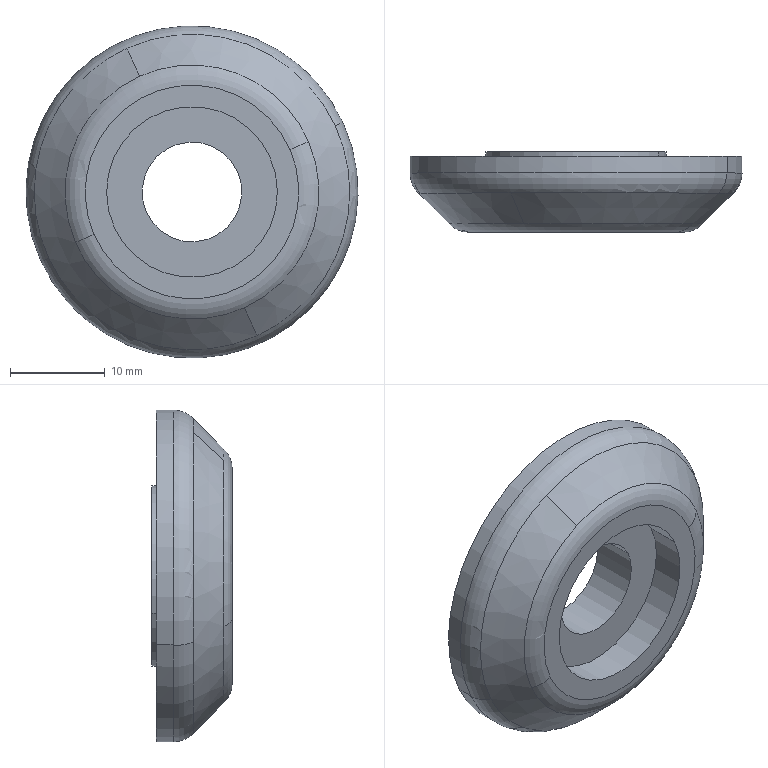Part | SolidWorks | features BaseBody 1 | 1 solid | 18 faces | box 35 x 8.5 x 35 mm | volume 5235 mm3 | cylinder 8 | torus 4 | plane 4 | cone 2 | commonest cylinder face diameters 10.5 x2 18 x2 19 x2 35 x2
STEP:
#1=CARTESIAN_POINT('',(-397.851,-130.5,38.987));
#2=VERTEX_POINT('',#1);
#3=CARTESIAN_POINT('',(-377.198,-130.5,47.953));
#4=VERTEX_POINT('',#3);
#5=CARTESIAN_POINT('',(-387.524,-130.5,43.47));
#6=DIRECTION('',(0.,-1.,0.));
#7=DIRECTION('',(-0.9114,0.,-0.4115));
#8=AXIS2_PLACEMENT_3D('',#5,#6,#7);
#9=CIRCLE('',#8,11.257);
#10=EDGE_CURVE('',#2,#4,#9,.T.);
#11=ORIENTED_EDGE('',*,*,#10,.F.);
#12=CARTESIAN_POINT('',(-399.797,-129.621,38.143));
#13=VERTEX_POINT('',#12);
#14=CARTESIAN_POINT('',(-397.851,-127.5,38.987));
#15=DIRECTION('',(0.3982,0.,-0.9173));
#16=DIRECTION('',(-0.9173,0.,-0.3982));
#17=AXIS2_PLACEMENT_3D('',#14,#15,#16);
#18=CIRCLE('',#17,3.);
#19=EDGE_CURVE('',#2,#13,#18,.T.);
#20=ORIENTED_EDGE('',*,*,#19,.T.);
#21=CARTESIAN_POINT('',(-382.019,-129.621,31.277));
#22=VERTEX_POINT('',#21);
#23=CARTESIAN_POINT('',(-387.524,-129.621,43.47));
#24=DIRECTION('',(0.,-1.,0.));
#25=DIRECTION('',(-0.9114,0.,-0.4115));
#26=AXIS2_PLACEMENT_3D('',#23,#24,#25);
#27=CIRCLE('',#26,13.379);
#28=EDGE_CURVE('',#13,#22,#27,.T.);
#29=ORIENTED_EDGE('',*,*,#28,.T.);
#30=CARTESIAN_POINT('',(-375.252,-129.621,48.797));
#31=VERTEX_POINT('',#30);
#32=CARTESIAN_POINT('',(-387.524,-129.621,43.47));
#33=DIRECTION('',(0.,-1.,0.));
#34=DIRECTION('',(-0.9114,0.,-0.4115));
#35=AXIS2_PLACEMENT_3D('',#32,#33,#34);
#36=CIRCLE('',#35,13.379);
#37=EDGE_CURVE('',#22,#31,#36,.T.);
#38=ORIENTED_EDGE('',*,*,#37,.T.);
#39=CARTESIAN_POINT('',(-377.198,-127.5,47.953));
#40=DIRECTION('',(-0.3982,0.,0.9173));
#41=DIRECTION('',(0.9173,0.,0.3982));
#42=AXIS2_PLACEMENT_3D('',#39,#40,#41);
#43=CIRCLE('',#42,3.);
#44=EDGE_CURVE('',#4,#31,#43,.T.);
#45=ORIENTED_EDGE('',*,*,#44,.F.);
#46=EDGE_LOOP('',(#11,#20,#29,#38,#45));
#47=FACE_OUTER_BOUND('',#46,.T.);
#48=CARTESIAN_POINT('',(-387.524,-127.5,43.47));
#49=DIRECTION('',(0.,1.,0.));
#50=DIRECTION('',(0.9173,0.,0.3982));
#51=AXIS2_PLACEMENT_3D('',#48,#49,#50);
#52=TOROIDAL_SURFACE('',#51,11.257,3.);
#53=ADVANCED_FACE('',(#47),#52,.T.);
#54=ORIENTED_EDGE('',*,*,#37,.F.);
#55=CARTESIAN_POINT('',(-380.685,-126.379,28.321));
#56=VERTEX_POINT('',#55);
#57=CARTESIAN_POINT('',(-381.352,-128.,29.799));
#58=DIRECTION('',(0.291,0.7071,-0.6445));
#59=VECTOR('',#58,1000.);
#60=LINE('',#57,#59);
#61=EDGE_CURVE('',#22,#56,#60,.T.);
#62=ORIENTED_EDGE('',*,*,#61,.T.);
#63=CARTESIAN_POINT('',(-372.434,-126.379,50.438));
#64=VERTEX_POINT('',#63);
#65=CARTESIAN_POINT('',(-387.524,-126.379,43.47));
#66=DIRECTION('',(0.,1.,0.));
#67=DIRECTION('',(-0.9114,0.,-0.4115));
#68=AXIS2_PLACEMENT_3D('',#65,#66,#67);
#69=CIRCLE('',#68,16.621);
#70=EDGE_CURVE('',#64,#56,#69,.T.);
#71=ORIENTED_EDGE('',*,*,#70,.F.);
#72=CARTESIAN_POINT('',(-394.364,-126.379,58.619));
#73=VERTEX_POINT('',#72);
#74=CARTESIAN_POINT('',(-387.524,-126.379,43.47));
#75=DIRECTION('',(0.,1.,0.));
#76=DIRECTION('',(-0.9114,0.,-0.4115));
#77=AXIS2_PLACEMENT_3D('',#74,#75,#76);
#78=CIRCLE('',#77,16.621);
#79=EDGE_CURVE('',#73,#64,#78,.T.);
#80=ORIENTED_EDGE('',*,*,#79,.F.);
#81=CARTESIAN_POINT('',(-393.03,-129.621,55.663));
#82=VERTEX_POINT('',#81);
#83=CARTESIAN_POINT('',(-393.697,-128.,57.141));
#84=DIRECTION('',(-0.291,0.7071,0.6445));
#85=VECTOR('',#84,1000.);
#86=LINE('',#83,#85);
#87=EDGE_CURVE('',#82,#73,#86,.T.);
#88=ORIENTED_EDGE('',*,*,#87,.F.);
#89=CARTESIAN_POINT('',(-387.524,-129.621,43.47));
#90=DIRECTION('',(0.,-1.,0.));
#91=DIRECTION('',(-0.9114,0.,-0.4115));
#92=AXIS2_PLACEMENT_3D('',#89,#90,#91);
#93=CIRCLE('',#92,13.379);
#94=EDGE_CURVE('',#31,#82,#93,.T.);
#95=ORIENTED_EDGE('',*,*,#94,.F.);
#96=EDGE_LOOP('',(#54,#62,#71,#80,#88,#95));
#97=FACE_OUTER_BOUND('',#96,.T.);
#98=CARTESIAN_POINT('',(-387.524,-128.,43.47));
#99=DIRECTION('',(0.,1.,0.));
#100=DIRECTION('',(-0.4115,0.,0.9114));
#101=AXIS2_PLACEMENT_3D('',#98,#99,#100);
#102=CONICAL_SURFACE('',#101,15.,0.7854);
#103=ADVANCED_FACE('',(#97),#102,.T.);
#104=CARTESIAN_POINT('',(-371.636,-124.257,50.806));
#105=VERTEX_POINT('',#104);
#106=CARTESIAN_POINT('',(-371.575,-124.257,50.672));
#107=VERTEX_POINT('',#106);
#108=CARTESIAN_POINT('',(-387.524,-124.257,43.47));
#109=DIRECTION('',(0.,1.,0.));
#110=DIRECTION('',(0.9114,0.,0.4115));
#111=AXIS2_PLACEMENT_3D('',#108,#109,#110);
#112=CIRCLE('',#111,17.5);
#113=EDGE_CURVE('',#105,#107,#112,.T.);
#114=ORIENTED_EDGE('',*,*,#113,.F.);
#115=CARTESIAN_POINT('',(-374.36,-124.257,49.548));
#116=DIRECTION('',(0.4192,0.,-0.9079));
#117=DIRECTION('',(-0.9079,0.,-0.4192));
#118=AXIS2_PLACEMENT_3D('',#115,#116,#117);
#119=CIRCLE('',#118,3.);
#120=EDGE_CURVE('',#105,#64,#119,.T.);
#121=ORIENTED_EDGE('',*,*,#120,.T.);
#122=ORIENTED_EDGE('',*,*,#70,.T.);
#123=CARTESIAN_POINT('',(-402.615,-126.379,36.502));
#124=VERTEX_POINT('',#123);
#125=CARTESIAN_POINT('',(-387.524,-126.379,43.47));
#126=DIRECTION('',(0.,1.,0.));
#127=DIRECTION('',(-0.9114,0.,-0.4115));
#128=AXIS2_PLACEMENT_3D('',#125,#126,#127);
#129=CIRCLE('',#128,16.621);
#130=EDGE_CURVE('',#56,#124,#129,.T.);
#131=ORIENTED_EDGE('',*,*,#130,.T.);
#132=CARTESIAN_POINT('',(-403.413,-124.257,36.134));
#133=VERTEX_POINT('',#132);
#134=CARTESIAN_POINT('',(-400.689,-124.257,37.392));
#135=DIRECTION('',(-0.4192,0.,0.9079));
#136=DIRECTION('',(0.9079,0.,0.4192));
#137=AXIS2_PLACEMENT_3D('',#134,#135,#136);
#138=CIRCLE('',#137,3.);
#139=EDGE_CURVE('',#133,#124,#138,.T.);
#140=ORIENTED_EDGE('',*,*,#139,.F.);
#141=CARTESIAN_POINT('',(-387.524,-124.257,43.47));
#142=DIRECTION('',(0.,1.,0.));
#143=DIRECTION('',(0.9114,0.,0.4115));
#144=AXIS2_PLACEMENT_3D('',#141,#142,#143);
#145=CIRCLE('',#144,17.5);
#146=EDGE_CURVE('',#107,#133,#145,.T.);
#147=ORIENTED_EDGE('',*,*,#146,.F.);
#148=EDGE_LOOP('',(#114,#121,#122,#131,#140,#147));
#149=FACE_OUTER_BOUND('',#148,.T.);
#150=CARTESIAN_POINT('',(-387.524,-124.257,43.47));
#151=DIRECTION('',(0.,-1.,0.));
#152=DIRECTION('',(-0.9079,0.,-0.4192));
#153=AXIS2_PLACEMENT_3D('',#150,#151,#152);
#154=TOROIDAL_SURFACE('',#153,14.5,3.);
#155=ADVANCED_FACE('',(#149),#154,.T.);
#156=CARTESIAN_POINT('',(-392.309,-122.,41.31));
#157=VERTEX_POINT('',#156);
#158=CARTESIAN_POINT('',(-382.74,-122.,45.631));
#159=VERTEX_POINT('',#158);
#160=CARTESIAN_POINT('',(-387.524,-122.,43.47));
#161=DIRECTION('',(0.,1.,0.));
#162=DIRECTION('',(-0.9114,0.,-0.4115));
#163=AXIS2_PLACEMENT_3D('',#160,#161,#162);
#164=CIRCLE('',#163,5.25);
#165=EDGE_CURVE('',#157,#159,#164,.T.);
#166=ORIENTED_EDGE('',*,*,#165,.T.);
#167=CARTESIAN_POINT('',(-382.74,-127.,45.631));
#168=VERTEX_POINT('',#167);
#169=CARTESIAN_POINT('',(-382.74,-122.,45.631));
#170=DIRECTION('',(0.,-1.,0.));
#171=VECTOR('',#170,1000.);
#172=LINE('',#169,#171);
#173=EDGE_CURVE('',#159,#168,#172,.T.);
#174=ORIENTED_EDGE('',*,*,#173,.T.);
#175=CARTESIAN_POINT('',(-392.309,-127.,41.31));
#176=VERTEX_POINT('',#175);
#177=CARTESIAN_POINT('',(-387.524,-127.,43.47));
#178=DIRECTION('',(0.,-1.,0.));
#179=DIRECTION('',(0.9114,0.,0.4115));
#180=AXIS2_PLACEMENT_3D('',#177,#178,#179);
#181=CIRCLE('',#180,5.25);
#182=EDGE_CURVE('',#168,#176,#181,.T.);
#183=ORIENTED_EDGE('',*,*,#182,.T.);
#184=CARTESIAN_POINT('',(-392.309,-122.,41.31));
#185=DIRECTION('',(0.,-1.,0.));
#186=VECTOR('',#185,1000.);
#187=LINE('',#184,#186);
#188=EDGE_CURVE('',#157,#176,#187,.T.);
#189=ORIENTED_EDGE('',*,*,#188,.F.);
#190=EDGE_LOOP('',(#166,#174,#183,#189));
#191=FACE_OUTER_BOUND('',#190,.T.);
#192=CARTESIAN_POINT('',(-387.524,-122.,43.47));
#193=DIRECTION('',(0.,-1.,0.));
#194=DIRECTION('',(-0.9114,0.,-0.4115));
#195=AXIS2_PLACEMENT_3D('',#192,#193,#194);
#196=CYLINDRICAL_SURFACE('',#195,5.25);
#197=ADVANCED_FACE('',(#191),#196,.F.);
#198=CARTESIAN_POINT('',(-396.183,-122.,39.561));
#199=VERTEX_POINT('',#198);
#200=CARTESIAN_POINT('',(-378.866,-122.,47.379));
#201=VERTEX_POINT('',#200);
#202=CARTESIAN_POINT('',(-387.524,-122.,43.47));
#203=DIRECTION('',(0.,-1.,0.));
#204=DIRECTION('',(-0.9114,0.,-0.4115));
#205=AXIS2_PLACEMENT_3D('',#202,#203,#204);
#206=CIRCLE('',#205,9.5);
#207=EDGE_CURVE('',#199,#201,#206,.T.);
#208=ORIENTED_EDGE('',*,*,#207,.T.);
#209=CARTESIAN_POINT('',(-378.866,-122.5,47.379));
#210=VERTEX_POINT('',#209);
#211=CARTESIAN_POINT('',(-378.866,-122.,47.379));
#212=DIRECTION('',(0.,-1.,0.));
#213=VECTOR('',#212,1000.);
#214=LINE('',#211,#213);
#215=EDGE_CURVE('',#201,#210,#214,.T.);
#216=ORIENTED_EDGE('',*,*,#215,.T.);
#217=CARTESIAN_POINT('',(-396.183,-122.5,39.561));
#218=VERTEX_POINT('',#217);
#219=CARTESIAN_POINT('',(-387.524,-122.5,43.47));
#220=DIRECTION('',(0.,-1.,0.));
#221=DIRECTION('',(-0.9114,0.,-0.4115));
#222=AXIS2_PLACEMENT_3D('',#219,#220,#221);
#223=CIRCLE('',#222,9.5);
#224=EDGE_CURVE('',#218,#210,#223,.T.);
#225=ORIENTED_EDGE('',*,*,#224,.F.);
#226=CARTESIAN_POINT('',(-396.183,-122.,39.561));
#227=DIRECTION('',(0.,-1.,0.));
#228=VECTOR('',#227,1000.);
#229=LINE('',#226,#228);
#230=EDGE_CURVE('',#199,#218,#229,.T.);
#231=ORIENTED_EDGE('',*,*,#230,.F.);
#232=EDGE_LOOP('',(#208,#216,#225,#231));
#233=FACE_OUTER_BOUND('',#232,.T.);
#234=CARTESIAN_POINT('',(-387.524,-122.,43.47));
#235=DIRECTION('',(0.,-1.,0.));
#236=DIRECTION('',(-0.9114,0.,-0.4115));
#237=AXIS2_PLACEMENT_3D('',#234,#235,#236);
#238=CYLINDRICAL_SURFACE('',#237,9.5);
#239=ADVANCED_FACE('',(#233),#238,.T.);
#240=CARTESIAN_POINT('',(-403.474,-122.5,36.269));
#241=VERTEX_POINT('',#240);
#242=CARTESIAN_POINT('',(-371.575,-122.5,50.672));
#243=VERTEX_POINT('',#242);
#244=CARTESIAN_POINT('',(-387.524,-122.5,43.47));
#245=DIRECTION('',(0.,-1.,0.));
#246=DIRECTION('',(-0.9114,0.,-0.4115));
#247=AXIS2_PLACEMENT_3D('',#244,#245,#246);
#248=CIRCLE('',#247,17.5);
#249=EDGE_CURVE('',#241,#243,#248,.T.);
#250=ORIENTED_EDGE('',*,*,#249,.T.);
#251=CARTESIAN_POINT('',(-371.575,-122.5,50.672));
#252=DIRECTION('',(0.,-1.,0.));
#253=VECTOR('',#252,1000.);
#254=LINE('',#251,#253);
#255=EDGE_CURVE('',#243,#107,#254,.T.);
#256=ORIENTED_EDGE('',*,*,#255,.T.);
#257=ORIENTED_EDGE('',*,*,#146,.T.);
#258=CARTESIAN_POINT('',(-403.474,-124.257,36.269));
#259=VERTEX_POINT('',#258);
#260=CARTESIAN_POINT('',(-387.524,-124.257,43.47));
#261=DIRECTION('',(0.,1.,0.));
#262=DIRECTION('',(0.9114,0.,0.4115));
#263=AXIS2_PLACEMENT_3D('',#260,#261,#262);
#264=CIRCLE('',#263,17.5);
#265=EDGE_CURVE('',#133,#259,#264,.T.);
#266=ORIENTED_EDGE('',*,*,#265,.T.);
#267=CARTESIAN_POINT('',(-403.474,-122.5,36.269));
#268=DIRECTION('',(0.,-1.,0.));
#269=VECTOR('',#268,1000.);
#270=LINE('',#267,#269);
#271=EDGE_CURVE('',#241,#259,#270,.T.);
#272=ORIENTED_EDGE('',*,*,#271,.F.);
#273=EDGE_LOOP('',(#250,#256,#257,#266,#272));
#274=FACE_OUTER_BOUND('',#273,.T.);
#275=CARTESIAN_POINT('',(-387.524,-122.5,43.47));
#276=DIRECTION('',(0.,-1.,0.));
#277=DIRECTION('',(-0.9114,0.,-0.4115));
#278=AXIS2_PLACEMENT_3D('',#275,#276,#277);
#279=CYLINDRICAL_SURFACE('',#278,17.5);
#280=ADVANCED_FACE('',(#274),#279,.T.);
#281=CARTESIAN_POINT('',(-379.322,-127.,47.174));
#282=VERTEX_POINT('',#281);
#283=CARTESIAN_POINT('',(-395.727,-127.,39.766));
#284=VERTEX_POINT('',#283);
#285=CARTESIAN_POINT('',(-387.524,-127.,43.47));
#286=DIRECTION('',(0.,-1.,0.));
#287=DIRECTION('',(-0.9114,0.,-0.4115));
#288=AXIS2_PLACEMENT_3D('',#285,#286,#287);
#289=CIRCLE('',#288,9.);
#290=EDGE_CURVE('',#282,#284,#289,.T.);
#291=ORIENTED_EDGE('',*,*,#290,.F.);
#292=CARTESIAN_POINT('',(-379.322,-130.5,47.174));
#293=VERTEX_POINT('',#292);
#294=CARTESIAN_POINT('',(-379.322,-130.5,47.174));
#295=DIRECTION('',(0.,-1.,0.));
#296=VECTOR('',#295,1000.);
#297=LINE('',#294,#296);
#298=EDGE_CURVE('',#282,#293,#297,.T.);
#299=ORIENTED_EDGE('',*,*,#298,.T.);
#300=CARTESIAN_POINT('',(-395.727,-130.5,39.766));
#301=VERTEX_POINT('',#300);
#302=CARTESIAN_POINT('',(-387.524,-130.5,43.47));
#303=DIRECTION('',(0.,-1.,0.));
#304=DIRECTION('',(-0.9114,0.,-0.4115));
#305=AXIS2_PLACEMENT_3D('',#302,#303,#304);
#306=CIRCLE('',#305,9.);
#307=EDGE_CURVE('',#293,#301,#306,.T.);
#308=ORIENTED_EDGE('',*,*,#307,.T.);
#309=CARTESIAN_POINT('',(-395.727,-130.5,39.766));
#310=DIRECTION('',(0.,-1.,0.));
#311=VECTOR('',#310,1000.);
#312=LINE('',#309,#311);
#313=EDGE_CURVE('',#284,#301,#312,.T.);
#314=ORIENTED_EDGE('',*,*,#313,.F.);
#315=EDGE_LOOP('',(#291,#299,#308,#314));
#316=FACE_OUTER_BOUND('',#315,.T.);
#317=CARTESIAN_POINT('',(-387.524,-130.5,43.47));
#318=DIRECTION('',(0.,-1.,0.));
#319=DIRECTION('',(-0.9114,0.,-0.4115));
#320=AXIS2_PLACEMENT_3D('',#317,#318,#319);
#321=CYLINDRICAL_SURFACE('',#320,9.);
#322=ADVANCED_FACE('',(#316),#321,.F.);
#323=ORIENTED_EDGE('',*,*,#165,.F.);
#324=CARTESIAN_POINT('',(-387.524,-122.,43.47));
#325=DIRECTION('',(0.,1.,0.));
#326=DIRECTION('',(-0.9114,0.,-0.4115));
#327=AXIS2_PLACEMENT_3D('',#324,#325,#326);
#328=CIRCLE('',#327,5.25);
#329=EDGE_CURVE('',#159,#157,#328,.T.);
#330=ORIENTED_EDGE('',*,*,#329,.F.);
#331=EDGE_LOOP('',(#323,#330));
#332=FACE_BOUND('',#331,.T.);
#333=ORIENTED_EDGE('',*,*,#207,.F.);
#334=CARTESIAN_POINT('',(-387.524,-122.,43.47));
#335=DIRECTION('',(0.,-1.,0.));
#336=DIRECTION('',(-0.9114,0.,-0.4115));
#337=AXIS2_PLACEMENT_3D('',#334,#335,#336);
#338=CIRCLE('',#337,9.5);
#339=EDGE_CURVE('',#201,#199,#338,.T.);
#340=ORIENTED_EDGE('',*,*,#339,.F.);
#341=EDGE_LOOP('',(#333,#340));
#342=FACE_OUTER_BOUND('',#341,.T.);
#343=CARTESIAN_POINT('',(-21.78,-122.,172.659));
#344=DIRECTION('',(0.,-1.,0.));
#345=DIRECTION('',(0.,0.,-1.));
#346=AXIS2_PLACEMENT_3D('',#343,#344,#345);
#347=PLANE('',#346);
#348=ADVANCED_FACE('',(#332,#342),#347,.F.);
#349=CARTESIAN_POINT('',(-387.524,-127.,43.47));
#350=DIRECTION('',(0.,-1.,0.));
#351=DIRECTION('',(0.9114,0.,0.4115));
#352=AXIS2_PLACEMENT_3D('',#349,#350,#351);
#353=CIRCLE('',#352,5.25);
#354=EDGE_CURVE('',#176,#168,#353,.T.);
#355=ORIENTED_EDGE('',*,*,#354,.F.);
#356=ORIENTED_EDGE('',*,*,#182,.F.);
#357=EDGE_LOOP('',(#355,#356));
#358=FACE_BOUND('',#357,.T.);
#359=CARTESIAN_POINT('',(-387.524,-127.,43.47));
#360=DIRECTION('',(0.,-1.,0.));
#361=DIRECTION('',(-0.9114,0.,-0.4115));
#362=AXIS2_PLACEMENT_3D('',#359,#360,#361);
#363=CIRCLE('',#362,9.);
#364=EDGE_CURVE('',#284,#282,#363,.T.);
#365=ORIENTED_EDGE('',*,*,#364,.T.);
#366=ORIENTED_EDGE('',*,*,#290,.T.);
#367=EDGE_LOOP('',(#365,#366));
#368=FACE_OUTER_BOUND('',#367,.T.);
#369=CARTESIAN_POINT('',(-21.78,-127.,172.659));
#370=DIRECTION('',(0.,-1.,0.));
#371=DIRECTION('',(0.,0.,-1.));
#372=AXIS2_PLACEMENT_3D('',#369,#370,#371);
#373=PLANE('',#372);
#374=ADVANCED_FACE('',(#358,#368),#373,.T.);
#375=CARTESIAN_POINT('',(-387.524,-130.5,43.47));
#376=DIRECTION('',(0.,-1.,0.));
#377=DIRECTION('',(-0.9114,0.,-0.4115));
#378=AXIS2_PLACEMENT_3D('',#375,#376,#377);
#379=CIRCLE('',#378,9.);
#380=EDGE_CURVE('',#301,#293,#379,.T.);
#381=ORIENTED_EDGE('',*,*,#380,.F.);
#382=ORIENTED_EDGE('',*,*,#307,.F.);
#383=EDGE_LOOP('',(#381,#382));
#384=FACE_BOUND('',#383,.T.);
#385=CARTESIAN_POINT('',(-387.524,-130.5,43.47));
#386=DIRECTION('',(0.,-1.,0.));
#387=DIRECTION('',(-0.9114,0.,-0.4115));
#388=AXIS2_PLACEMENT_3D('',#385,#386,#387);
#389=CIRCLE('',#388,11.257);
#390=EDGE_CURVE('',#4,#2,#389,.T.);
#391=ORIENTED_EDGE('',*,*,#390,.T.);
#392=ORIENTED_EDGE('',*,*,#10,.T.);
#393=EDGE_LOOP('',(#391,#392));
#394=FACE_OUTER_BOUND('',#393,.T.);
#395=CARTESIAN_POINT('',(-21.78,-130.5,172.659));
#396=DIRECTION('',(0.,-1.,0.));
#397=DIRECTION('',(0.,0.,-1.));
#398=AXIS2_PLACEMENT_3D('',#395,#396,#397);
#399=PLANE('',#398);
#400=ADVANCED_FACE('',(#384,#394),#399,.T.);
#401=ORIENTED_EDGE('',*,*,#298,.F.);
#402=ORIENTED_EDGE('',*,*,#364,.F.);
#403=ORIENTED_EDGE('',*,*,#313,.T.);
#404=ORIENTED_EDGE('',*,*,#380,.T.);
#405=EDGE_LOOP('',(#401,#402,#403,#404));
#406=FACE_OUTER_BOUND('',#405,.T.);
#407=CARTESIAN_POINT('',(-387.524,-130.5,43.47));
#408=DIRECTION('',(0.,-1.,0.));
#409=DIRECTION('',(-0.9114,0.,-0.4115));
#410=AXIS2_PLACEMENT_3D('',#407,#408,#409);
#411=CYLINDRICAL_SURFACE('',#410,9.);
#412=ADVANCED_FACE('',(#406),#411,.F.);
#413=ORIENTED_EDGE('',*,*,#255,.F.);
#414=CARTESIAN_POINT('',(-387.524,-122.5,43.47));
#415=DIRECTION('',(0.,-1.,0.));
#416=DIRECTION('',(-0.9114,0.,-0.4115));
#417=AXIS2_PLACEMENT_3D('',#414,#415,#416);
#418=CIRCLE('',#417,17.5);
#419=EDGE_CURVE('',#243,#241,#418,.T.);
#420=ORIENTED_EDGE('',*,*,#419,.T.);
#421=ORIENTED_EDGE('',*,*,#271,.T.);
#422=CARTESIAN_POINT('',(-387.524,-124.257,43.47));
#423=DIRECTION('',(0.,1.,0.));
#424=DIRECTION('',(0.9114,0.,0.4115));
#425=AXIS2_PLACEMENT_3D('',#422,#423,#424);
#426=CIRCLE('',#425,17.5);
#427=EDGE_CURVE('',#259,#105,#426,.T.);
#428=ORIENTED_EDGE('',*,*,#427,.T.);
#429=ORIENTED_EDGE('',*,*,#113,.T.);
#430=EDGE_LOOP('',(#413,#420,#421,#428,#429));
#431=FACE_OUTER_BOUND('',#430,.T.);
#432=CARTESIAN_POINT('',(-387.524,-122.5,43.47));
#433=DIRECTION('',(0.,-1.,0.));
#434=DIRECTION('',(-0.9114,0.,-0.4115));
#435=AXIS2_PLACEMENT_3D('',#432,#433,#434);
#436=CYLINDRICAL_SURFACE('',#435,17.5);
#437=ADVANCED_FACE('',(#431),#436,.T.);
#438=ORIENTED_EDGE('',*,*,#224,.T.);
#439=CARTESIAN_POINT('',(-387.524,-122.5,43.47));
#440=DIRECTION('',(0.,-1.,0.));
#441=DIRECTION('',(-0.9114,0.,-0.4115));
#442=AXIS2_PLACEMENT_3D('',#439,#440,#441);
#443=CIRCLE('',#442,9.5);
#444=EDGE_CURVE('',#210,#218,#443,.T.);
#445=ORIENTED_EDGE('',*,*,#444,.T.);
#446=EDGE_LOOP('',(#438,#445));
#447=FACE_BOUND('',#446,.T.);
#448=ORIENTED_EDGE('',*,*,#249,.F.);
#449=ORIENTED_EDGE('',*,*,#419,.F.);
#450=EDGE_LOOP('',(#448,#449));
#451=FACE_OUTER_BOUND('',#450,.T.);
#452=CARTESIAN_POINT('',(-21.78,-122.5,172.659));
#453=DIRECTION('',(0.,-1.,0.));
#454=DIRECTION('',(0.,0.,-1.));
#455=AXIS2_PLACEMENT_3D('',#452,#453,#454);
#456=PLANE('',#455);
#457=ADVANCED_FACE('',(#447,#451),#456,.F.);
#458=ORIENTED_EDGE('',*,*,#215,.F.);
#459=ORIENTED_EDGE('',*,*,#339,.T.);
#460=ORIENTED_EDGE('',*,*,#230,.T.);
#461=ORIENTED_EDGE('',*,*,#444,.F.);
#462=EDGE_LOOP('',(#458,#459,#460,#461));
#463=FACE_OUTER_BOUND('',#462,.T.);
#464=CARTESIAN_POINT('',(-387.524,-122.,43.47));
#465=DIRECTION('',(0.,-1.,0.));
#466=DIRECTION('',(-0.9114,0.,-0.4115));
#467=AXIS2_PLACEMENT_3D('',#464,#465,#466);
#468=CYLINDRICAL_SURFACE('',#467,9.5);
#469=ADVANCED_FACE('',(#463),#468,.T.);
#470=ORIENTED_EDGE('',*,*,#173,.F.);
#471=ORIENTED_EDGE('',*,*,#329,.T.);
#472=ORIENTED_EDGE('',*,*,#188,.T.);
#473=ORIENTED_EDGE('',*,*,#354,.T.);
#474=EDGE_LOOP('',(#470,#471,#472,#473));
#475=FACE_OUTER_BOUND('',#474,.T.);
#476=CARTESIAN_POINT('',(-387.524,-122.,43.47));
#477=DIRECTION('',(0.,-1.,0.));
#478=DIRECTION('',(-0.9114,0.,-0.4115));
#479=AXIS2_PLACEMENT_3D('',#476,#477,#478);
#480=CYLINDRICAL_SURFACE('',#479,5.25);
#481=ADVANCED_FACE('',(#475),#480,.F.);
#482=ORIENTED_EDGE('',*,*,#120,.F.);
#483=ORIENTED_EDGE('',*,*,#427,.F.);
#484=ORIENTED_EDGE('',*,*,#265,.F.);
#485=ORIENTED_EDGE('',*,*,#139,.T.);
#486=CARTESIAN_POINT('',(-387.524,-126.379,43.47));
#487=DIRECTION('',(0.,1.,0.));
#488=DIRECTION('',(-0.9114,0.,-0.4115));
#489=AXIS2_PLACEMENT_3D('',#486,#487,#488);
#490=CIRCLE('',#489,16.621);
#491=EDGE_CURVE('',#124,#73,#490,.T.);
#492=ORIENTED_EDGE('',*,*,#491,.T.);
#493=ORIENTED_EDGE('',*,*,#79,.T.);
#494=EDGE_LOOP('',(#482,#483,#484,#485,#492,#493));
#495=FACE_OUTER_BOUND('',#494,.T.);
#496=CARTESIAN_POINT('',(-387.524,-124.257,43.47));
#497=DIRECTION('',(0.,-1.,0.));
#498=DIRECTION('',(-0.9079,0.,-0.4192));
#499=AXIS2_PLACEMENT_3D('',#496,#497,#498);
#500=TOROIDAL_SURFACE('',#499,14.5,3.);
#501=ADVANCED_FACE('',(#495),#500,.T.);
#502=ORIENTED_EDGE('',*,*,#61,.F.);
#503=ORIENTED_EDGE('',*,*,#28,.F.);
#504=CARTESIAN_POINT('',(-387.524,-129.621,43.47));
#505=DIRECTION('',(0.,-1.,0.));
#506=DIRECTION('',(-0.9114,0.,-0.4115));
#507=AXIS2_PLACEMENT_3D('',#504,#505,#506);
#508=CIRCLE('',#507,13.379);
#509=EDGE_CURVE('',#82,#13,#508,.T.);
#510=ORIENTED_EDGE('',*,*,#509,.F.);
#511=ORIENTED_EDGE('',*,*,#87,.T.);
#512=ORIENTED_EDGE('',*,*,#491,.F.);
#513=ORIENTED_EDGE('',*,*,#130,.F.);
#514=EDGE_LOOP('',(#502,#503,#510,#511,#512,#513));
#515=FACE_OUTER_BOUND('',#514,.T.);
#516=CARTESIAN_POINT('',(-387.524,-128.,43.47));
#517=DIRECTION('',(0.,1.,0.));
#518=DIRECTION('',(-0.4115,0.,0.9114));
#519=AXIS2_PLACEMENT_3D('',#516,#517,#518);
#520=CONICAL_SURFACE('',#519,15.,0.7854);
#521=ADVANCED_FACE('',(#515),#520,.T.);
#522=ORIENTED_EDGE('',*,*,#19,.F.);
#523=ORIENTED_EDGE('',*,*,#390,.F.);
#524=ORIENTED_EDGE('',*,*,#44,.T.);
#525=ORIENTED_EDGE('',*,*,#94,.T.);
#526=ORIENTED_EDGE('',*,*,#509,.T.);
#527=EDGE_LOOP('',(#522,#523,#524,#525,#526));
#528=FACE_OUTER_BOUND('',#527,.T.);
#529=CARTESIAN_POINT('',(-387.524,-127.5,43.47));
#530=DIRECTION('',(0.,1.,0.));
#531=DIRECTION('',(0.9173,0.,0.3982));
#532=AXIS2_PLACEMENT_3D('',#529,#530,#531);
#533=TOROIDAL_SURFACE('',#532,11.257,3.);
#534=ADVANCED_FACE('',(#528),#533,.T.);
#535=CLOSED_SHELL('',(#53,#103,#155,#197,#239,#280,#322,#348,#374,#400,#412,#437,#457,#469,#481,#501,#521,#534));
#536=MANIFOLD_SOLID_BREP('',#535);
#537=CARTESIAN_POINT('',(0.,0.,0.));
#538=DIRECTION('',(0.,0.,1.));
#539=DIRECTION('',(1.,0.,0.));
#540=AXIS2_PLACEMENT_3D('',#537,#538,#539);
#541=(LENGTH_UNIT()NAMED_UNIT(*)SI_UNIT(.MILLI.,.METRE.));
#542=UNCERTAINTY_MEASURE_WITH_UNIT(LENGTH_MEASURE(0.00001),#541,'','');
#543=(NAMED_UNIT(*)PLANE_ANGLE_UNIT()SI_UNIT($,.RADIAN.));
#544=(NAMED_UNIT(*)SI_UNIT($,.STERADIAN.)SOLID_ANGLE_UNIT());
#545=(GEOMETRIC_REPRESENTATION_CONTEXT(3)GLOBAL_UNCERTAINTY_ASSIGNED_CONTEXT((#542))GLOBAL_UNIT_ASSIGNED_CONTEXT((#541,#543,#544))REPRESENTATION_CONTEXT('',''));
#546=ADVANCED_BREP_SHAPE_REPRESENTATION('',(#536,#540),#545);